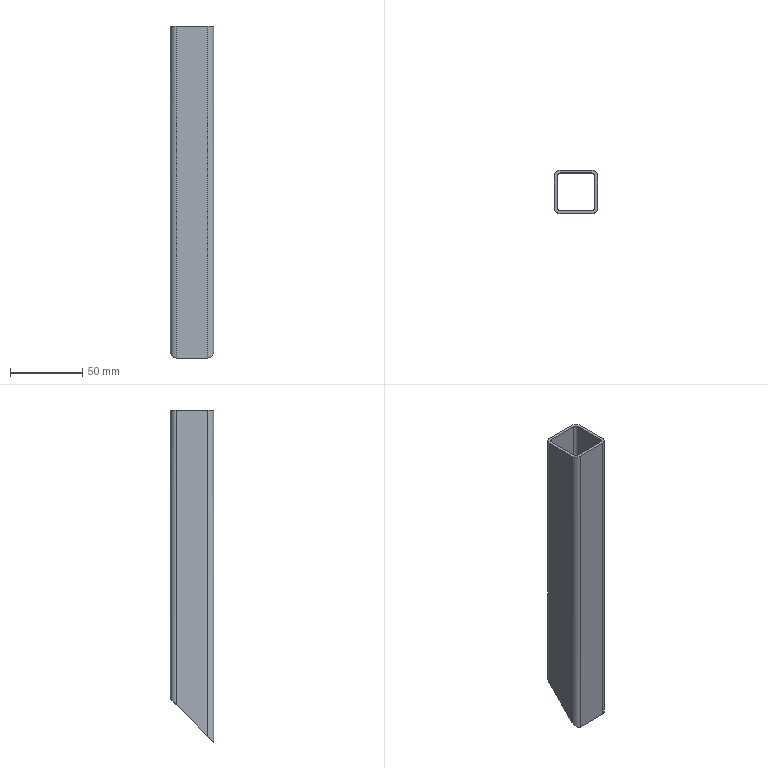Part | NX | features DATUM_CSYS 3, EXTRUDE 2, SKETCH 2, CPROJ 1 | 1 solid | 18 faces | box 30 x 30 x 230 mm | volume 45945 mm3 | plane 10 | cylinder 8 | commonest cylinder face diameters 4 x4 8 x4
STEP:
#1=CARTESIAN_POINT('',(15.,11.,230.));
#2=VERTEX_POINT('',#1);
#3=CARTESIAN_POINT('',(11.,15.,230.));
#4=VERTEX_POINT('',#3);
#5=CARTESIAN_POINT('',(11.,11.,230.));
#6=DIRECTION('',(0.,0.,1.));
#7=DIRECTION('',(1.,0.,0.));
#8=AXIS2_PLACEMENT_3D('',#5,#6,#7);
#9=CIRCLE('',#8,4.);
#10=EDGE_CURVE('',#2,#4,#9,.T.);
#11=ORIENTED_EDGE('',*,*,#10,.T.);
#12=CARTESIAN_POINT('',(-11.,15.,230.));
#13=VERTEX_POINT('',#12);
#14=CARTESIAN_POINT('',(11.,15.,230.));
#15=DIRECTION('',(-1.,0.,0.));
#16=VECTOR('',#15,1000.);
#17=LINE('',#14,#16);
#18=EDGE_CURVE('',#4,#13,#17,.T.);
#19=ORIENTED_EDGE('',*,*,#18,.T.);
#20=CARTESIAN_POINT('',(-15.,11.,230.));
#21=VERTEX_POINT('',#20);
#22=CARTESIAN_POINT('',(-11.,11.,230.));
#23=DIRECTION('',(0.,0.,1.));
#24=DIRECTION('',(1.,0.,0.));
#25=AXIS2_PLACEMENT_3D('',#22,#23,#24);
#26=CIRCLE('',#25,4.);
#27=EDGE_CURVE('',#13,#21,#26,.T.);
#28=ORIENTED_EDGE('',*,*,#27,.T.);
#29=CARTESIAN_POINT('',(-15.,-11.,230.));
#30=VERTEX_POINT('',#29);
#31=CARTESIAN_POINT('',(-15.,11.,230.));
#32=DIRECTION('',(0.,-1.,0.));
#33=VECTOR('',#32,1000.);
#34=LINE('',#31,#33);
#35=EDGE_CURVE('',#21,#30,#34,.T.);
#36=ORIENTED_EDGE('',*,*,#35,.T.);
#37=CARTESIAN_POINT('',(-11.,-15.,230.));
#38=VERTEX_POINT('',#37);
#39=CARTESIAN_POINT('',(-11.,-11.,230.));
#40=DIRECTION('',(0.,0.,1.));
#41=DIRECTION('',(1.,0.,0.));
#42=AXIS2_PLACEMENT_3D('',#39,#40,#41);
#43=CIRCLE('',#42,4.);
#44=EDGE_CURVE('',#30,#38,#43,.T.);
#45=ORIENTED_EDGE('',*,*,#44,.T.);
#46=CARTESIAN_POINT('',(11.,-15.,230.));
#47=VERTEX_POINT('',#46);
#48=CARTESIAN_POINT('',(-11.,-15.,230.));
#49=DIRECTION('',(1.,0.,0.));
#50=VECTOR('',#49,1000.);
#51=LINE('',#48,#50);
#52=EDGE_CURVE('',#38,#47,#51,.T.);
#53=ORIENTED_EDGE('',*,*,#52,.T.);
#54=CARTESIAN_POINT('',(15.,-11.,230.));
#55=VERTEX_POINT('',#54);
#56=CARTESIAN_POINT('',(11.,-11.,230.));
#57=DIRECTION('',(0.,0.,1.));
#58=DIRECTION('',(1.,0.,0.));
#59=AXIS2_PLACEMENT_3D('',#56,#57,#58);
#60=CIRCLE('',#59,4.);
#61=EDGE_CURVE('',#47,#55,#60,.T.);
#62=ORIENTED_EDGE('',*,*,#61,.T.);
#63=CARTESIAN_POINT('',(15.,-11.,230.));
#64=DIRECTION('',(0.,1.,0.));
#65=VECTOR('',#64,1000.);
#66=LINE('',#63,#65);
#67=EDGE_CURVE('',#55,#2,#66,.T.);
#68=ORIENTED_EDGE('',*,*,#67,.T.);
#69=EDGE_LOOP('',(#11,#19,#28,#36,#45,#53,#62,#68));
#70=FACE_BOUND('',#69,.T.);
#71=CARTESIAN_POINT('',(13.,11.,230.));
#72=VERTEX_POINT('',#71);
#73=CARTESIAN_POINT('',(11.,13.,230.));
#74=VERTEX_POINT('',#73);
#75=CARTESIAN_POINT('',(11.,11.,230.));
#76=DIRECTION('',(0.,0.,1.));
#77=DIRECTION('',(1.,0.,0.));
#78=AXIS2_PLACEMENT_3D('',#75,#76,#77);
#79=CIRCLE('',#78,2.);
#80=EDGE_CURVE('',#72,#74,#79,.T.);
#81=ORIENTED_EDGE('',*,*,#80,.F.);
#82=CARTESIAN_POINT('',(13.,-11.,230.));
#83=VERTEX_POINT('',#82);
#84=CARTESIAN_POINT('',(13.,-11.,230.));
#85=DIRECTION('',(0.,1.,0.));
#86=VECTOR('',#85,1000.);
#87=LINE('',#84,#86);
#88=EDGE_CURVE('',#83,#72,#87,.T.);
#89=ORIENTED_EDGE('',*,*,#88,.F.);
#90=CARTESIAN_POINT('',(11.,-13.,230.));
#91=VERTEX_POINT('',#90);
#92=CARTESIAN_POINT('',(11.,-11.,230.));
#93=DIRECTION('',(0.,0.,1.));
#94=DIRECTION('',(1.,0.,0.));
#95=AXIS2_PLACEMENT_3D('',#92,#93,#94);
#96=CIRCLE('',#95,2.);
#97=EDGE_CURVE('',#91,#83,#96,.T.);
#98=ORIENTED_EDGE('',*,*,#97,.F.);
#99=CARTESIAN_POINT('',(-11.,-13.,230.));
#100=VERTEX_POINT('',#99);
#101=CARTESIAN_POINT('',(-11.,-13.,230.));
#102=DIRECTION('',(1.,0.,0.));
#103=VECTOR('',#102,1000.);
#104=LINE('',#101,#103);
#105=EDGE_CURVE('',#100,#91,#104,.T.);
#106=ORIENTED_EDGE('',*,*,#105,.F.);
#107=CARTESIAN_POINT('',(-13.,-11.,230.));
#108=VERTEX_POINT('',#107);
#109=CARTESIAN_POINT('',(-11.,-11.,230.));
#110=DIRECTION('',(0.,0.,1.));
#111=DIRECTION('',(1.,0.,0.));
#112=AXIS2_PLACEMENT_3D('',#109,#110,#111);
#113=CIRCLE('',#112,2.);
#114=EDGE_CURVE('',#108,#100,#113,.T.);
#115=ORIENTED_EDGE('',*,*,#114,.F.);
#116=CARTESIAN_POINT('',(-13.,11.,230.));
#117=VERTEX_POINT('',#116);
#118=CARTESIAN_POINT('',(-13.,11.,230.));
#119=DIRECTION('',(0.,-1.,0.));
#120=VECTOR('',#119,1000.);
#121=LINE('',#118,#120);
#122=EDGE_CURVE('',#117,#108,#121,.T.);
#123=ORIENTED_EDGE('',*,*,#122,.F.);
#124=CARTESIAN_POINT('',(-11.,13.,230.));
#125=VERTEX_POINT('',#124);
#126=CARTESIAN_POINT('',(-11.,11.,230.));
#127=DIRECTION('',(0.,0.,1.));
#128=DIRECTION('',(1.,0.,0.));
#129=AXIS2_PLACEMENT_3D('',#126,#127,#128);
#130=CIRCLE('',#129,2.);
#131=EDGE_CURVE('',#125,#117,#130,.T.);
#132=ORIENTED_EDGE('',*,*,#131,.F.);
#133=CARTESIAN_POINT('',(11.,13.,230.));
#134=DIRECTION('',(-1.,0.,0.));
#135=VECTOR('',#134,1000.);
#136=LINE('',#133,#135);
#137=EDGE_CURVE('',#74,#125,#136,.T.);
#138=ORIENTED_EDGE('',*,*,#137,.F.);
#139=EDGE_LOOP('',(#81,#89,#98,#106,#115,#123,#132,#138));
#140=FACE_BOUND('',#139,.T.);
#141=CARTESIAN_POINT('',(11.,11.,230.));
#142=DIRECTION('',(0.,0.,-1.));
#143=DIRECTION('',(-1.,0.,0.));
#144=AXIS2_PLACEMENT_3D('',#141,#142,#143);
#145=PLANE('',#144);
#146=ADVANCED_FACE('',(#70,#140),#145,.F.);
#147=CARTESIAN_POINT('',(-11.,15.,30.));
#148=VERTEX_POINT('',#147);
#149=CARTESIAN_POINT('',(11.,15.,30.));
#150=VERTEX_POINT('',#149);
#151=CARTESIAN_POINT('',(-29.5,15.,30.));
#152=DIRECTION('',(1.,0.,0.));
#153=VECTOR('',#152,1000.);
#154=LINE('',#151,#153);
#155=EDGE_CURVE('',#148,#150,#154,.T.);
#156=ORIENTED_EDGE('',*,*,#155,.F.);
#157=CARTESIAN_POINT('',(-11.,15.,0.));
#158=DIRECTION('',(0.,0.,1.));
#159=VECTOR('',#158,1000.);
#160=LINE('',#157,#159);
#161=EDGE_CURVE('',#148,#13,#160,.T.);
#162=ORIENTED_EDGE('',*,*,#161,.T.);
#163=ORIENTED_EDGE('',*,*,#18,.F.);
#164=CARTESIAN_POINT('',(11.,15.,0.));
#165=DIRECTION('',(0.,0.,1.));
#166=VECTOR('',#165,1000.);
#167=LINE('',#164,#166);
#168=EDGE_CURVE('',#150,#4,#167,.T.);
#169=ORIENTED_EDGE('',*,*,#168,.F.);
#170=EDGE_LOOP('',(#156,#162,#163,#169));
#171=FACE_BOUND('',#170,.T.);
#172=CARTESIAN_POINT('',(11.,15.,0.));
#173=DIRECTION('',(0.,1.,0.));
#174=DIRECTION('',(-1.,0.,0.));
#175=AXIS2_PLACEMENT_3D('',#172,#173,#174);
#176=PLANE('',#175);
#177=ADVANCED_FACE('',(#171),#176,.T.);
#178=CARTESIAN_POINT('',(-15.,11.,26.));
#179=VERTEX_POINT('',#178);
#180=CARTESIAN_POINT('',(-11.,11.,26.));
#181=DIRECTION('',(0.,-0.7071,0.7071));
#182=DIRECTION('',(0.,0.7071,0.7071));
#183=AXIS2_PLACEMENT_3D('',#180,#181,#182);
#184=ELLIPSE('',#183,5.657,4.);
#185=EDGE_CURVE('',#179,#148,#184,.F.);
#186=ORIENTED_EDGE('',*,*,#185,.F.);
#187=CARTESIAN_POINT('',(-15.,11.,0.));
#188=DIRECTION('',(0.,0.,1.));
#189=VECTOR('',#188,1000.);
#190=LINE('',#187,#189);
#191=EDGE_CURVE('',#179,#21,#190,.T.);
#192=ORIENTED_EDGE('',*,*,#191,.T.);
#193=ORIENTED_EDGE('',*,*,#27,.F.);
#194=ORIENTED_EDGE('',*,*,#161,.F.);
#195=EDGE_LOOP('',(#186,#192,#193,#194));
#196=FACE_BOUND('',#195,.T.);
#197=CARTESIAN_POINT('',(-11.,11.,0.));
#198=DIRECTION('',(0.,0.,1.));
#199=DIRECTION('',(1.,0.,0.));
#200=AXIS2_PLACEMENT_3D('',#197,#198,#199);
#201=CYLINDRICAL_SURFACE('',#200,4.);
#202=ADVANCED_FACE('',(#196),#201,.T.);
#203=CARTESIAN_POINT('',(-15.,-11.,4.));
#204=VERTEX_POINT('',#203);
#205=CARTESIAN_POINT('',(-15.,-2.,13.));
#206=DIRECTION('',(0.,0.7071,0.7071));
#207=VECTOR('',#206,1000.);
#208=LINE('',#205,#207);
#209=EDGE_CURVE('',#204,#179,#208,.T.);
#210=ORIENTED_EDGE('',*,*,#209,.F.);
#211=CARTESIAN_POINT('',(-15.,-11.,0.));
#212=DIRECTION('',(0.,0.,1.));
#213=VECTOR('',#212,1000.);
#214=LINE('',#211,#213);
#215=EDGE_CURVE('',#204,#30,#214,.T.);
#216=ORIENTED_EDGE('',*,*,#215,.T.);
#217=ORIENTED_EDGE('',*,*,#35,.F.);
#218=ORIENTED_EDGE('',*,*,#191,.F.);
#219=EDGE_LOOP('',(#210,#216,#217,#218));
#220=FACE_BOUND('',#219,.T.);
#221=CARTESIAN_POINT('',(-15.,11.,0.));
#222=DIRECTION('',(-1.,0.,0.));
#223=DIRECTION('',(0.,-1.,0.));
#224=AXIS2_PLACEMENT_3D('',#221,#222,#223);
#225=PLANE('',#224);
#226=ADVANCED_FACE('',(#220),#225,.T.);
#227=CARTESIAN_POINT('',(-11.,-15.,0.));
#228=VERTEX_POINT('',#227);
#229=CARTESIAN_POINT('',(-11.,-11.,4.));
#230=DIRECTION('',(0.,-0.7071,0.7071));
#231=DIRECTION('',(0.,0.7071,0.7071));
#232=AXIS2_PLACEMENT_3D('',#229,#230,#231);
#233=ELLIPSE('',#232,5.657,4.);
#234=EDGE_CURVE('',#228,#204,#233,.F.);
#235=ORIENTED_EDGE('',*,*,#234,.F.);
#236=CARTESIAN_POINT('',(-11.,-15.,0.));
#237=DIRECTION('',(0.,0.,1.));
#238=VECTOR('',#237,1000.);
#239=LINE('',#236,#238);
#240=EDGE_CURVE('',#228,#38,#239,.T.);
#241=ORIENTED_EDGE('',*,*,#240,.T.);
#242=ORIENTED_EDGE('',*,*,#44,.F.);
#243=ORIENTED_EDGE('',*,*,#215,.F.);
#244=EDGE_LOOP('',(#235,#241,#242,#243));
#245=FACE_BOUND('',#244,.T.);
#246=CARTESIAN_POINT('',(-11.,-11.,0.));
#247=DIRECTION('',(0.,0.,1.));
#248=DIRECTION('',(1.,0.,0.));
#249=AXIS2_PLACEMENT_3D('',#246,#247,#248);
#250=CYLINDRICAL_SURFACE('',#249,4.);
#251=ADVANCED_FACE('',(#245),#250,.T.);
#252=ORIENTED_EDGE('',*,*,#52,.F.);
#253=ORIENTED_EDGE('',*,*,#240,.F.);
#254=CARTESIAN_POINT('',(11.,-15.,0.));
#255=VERTEX_POINT('',#254);
#256=CARTESIAN_POINT('',(-11.,-15.,0.));
#257=DIRECTION('',(1.,0.,0.));
#258=VECTOR('',#257,1000.);
#259=LINE('',#256,#258);
#260=EDGE_CURVE('',#228,#255,#259,.T.);
#261=ORIENTED_EDGE('',*,*,#260,.T.);
#262=CARTESIAN_POINT('',(11.,-15.,0.));
#263=DIRECTION('',(0.,0.,1.));
#264=VECTOR('',#263,1000.);
#265=LINE('',#262,#264);
#266=EDGE_CURVE('',#255,#47,#265,.T.);
#267=ORIENTED_EDGE('',*,*,#266,.T.);
#268=EDGE_LOOP('',(#252,#253,#261,#267));
#269=FACE_BOUND('',#268,.T.);
#270=CARTESIAN_POINT('',(-11.,-15.,0.));
#271=DIRECTION('',(0.,-1.,0.));
#272=DIRECTION('',(1.,0.,0.));
#273=AXIS2_PLACEMENT_3D('',#270,#271,#272);
#274=PLANE('',#273);
#275=ADVANCED_FACE('',(#269),#274,.T.);
#276=CARTESIAN_POINT('',(15.,-11.,4.));
#277=VERTEX_POINT('',#276);
#278=CARTESIAN_POINT('',(11.,-11.,4.));
#279=DIRECTION('',(0.,-0.7071,0.7071));
#280=DIRECTION('',(0.,0.7071,0.7071));
#281=AXIS2_PLACEMENT_3D('',#278,#279,#280);
#282=ELLIPSE('',#281,5.657,4.);
#283=EDGE_CURVE('',#277,#255,#282,.F.);
#284=ORIENTED_EDGE('',*,*,#283,.F.);
#285=CARTESIAN_POINT('',(15.,-11.,0.));
#286=DIRECTION('',(0.,0.,1.));
#287=VECTOR('',#286,1000.);
#288=LINE('',#285,#287);
#289=EDGE_CURVE('',#277,#55,#288,.T.);
#290=ORIENTED_EDGE('',*,*,#289,.T.);
#291=ORIENTED_EDGE('',*,*,#61,.F.);
#292=ORIENTED_EDGE('',*,*,#266,.F.);
#293=EDGE_LOOP('',(#284,#290,#291,#292));
#294=FACE_BOUND('',#293,.T.);
#295=CARTESIAN_POINT('',(11.,-11.,0.));
#296=DIRECTION('',(0.,0.,1.));
#297=DIRECTION('',(1.,0.,0.));
#298=AXIS2_PLACEMENT_3D('',#295,#296,#297);
#299=CYLINDRICAL_SURFACE('',#298,4.);
#300=ADVANCED_FACE('',(#294),#299,.T.);
#301=CARTESIAN_POINT('',(15.,11.,26.));
#302=VERTEX_POINT('',#301);
#303=CARTESIAN_POINT('',(15.,15.,30.));
#304=DIRECTION('',(0.,-0.7071,-0.7071));
#305=VECTOR('',#304,1000.);
#306=LINE('',#303,#305);
#307=EDGE_CURVE('',#302,#277,#306,.T.);
#308=ORIENTED_EDGE('',*,*,#307,.F.);
#309=CARTESIAN_POINT('',(15.,11.,0.));
#310=DIRECTION('',(0.,0.,1.));
#311=VECTOR('',#310,1000.);
#312=LINE('',#309,#311);
#313=EDGE_CURVE('',#302,#2,#312,.T.);
#314=ORIENTED_EDGE('',*,*,#313,.T.);
#315=ORIENTED_EDGE('',*,*,#67,.F.);
#316=ORIENTED_EDGE('',*,*,#289,.F.);
#317=EDGE_LOOP('',(#308,#314,#315,#316));
#318=FACE_BOUND('',#317,.T.);
#319=CARTESIAN_POINT('',(15.,-11.,0.));
#320=DIRECTION('',(1.,0.,0.));
#321=DIRECTION('',(0.,0.,-1.));
#322=AXIS2_PLACEMENT_3D('',#319,#320,#321);
#323=PLANE('',#322);
#324=ADVANCED_FACE('',(#318),#323,.T.);
#325=CARTESIAN_POINT('',(11.,11.,26.));
#326=DIRECTION('',(0.,-0.7071,0.7071));
#327=DIRECTION('',(0.,0.7071,0.7071));
#328=AXIS2_PLACEMENT_3D('',#325,#326,#327);
#329=ELLIPSE('',#328,5.657,4.);
#330=EDGE_CURVE('',#150,#302,#329,.F.);
#331=ORIENTED_EDGE('',*,*,#330,.F.);
#332=ORIENTED_EDGE('',*,*,#168,.T.);
#333=ORIENTED_EDGE('',*,*,#10,.F.);
#334=ORIENTED_EDGE('',*,*,#313,.F.);
#335=EDGE_LOOP('',(#331,#332,#333,#334));
#336=FACE_BOUND('',#335,.T.);
#337=CARTESIAN_POINT('',(11.,11.,0.));
#338=DIRECTION('',(0.,0.,1.));
#339=DIRECTION('',(1.,0.,0.));
#340=AXIS2_PLACEMENT_3D('',#337,#338,#339);
#341=CYLINDRICAL_SURFACE('',#340,4.);
#342=ADVANCED_FACE('',(#336),#341,.T.);
#343=CARTESIAN_POINT('',(-11.,13.,28.));
#344=VERTEX_POINT('',#343);
#345=CARTESIAN_POINT('',(-11.,13.,0.));
#346=DIRECTION('',(0.,0.,1.));
#347=VECTOR('',#346,1000.);
#348=LINE('',#345,#347);
#349=EDGE_CURVE('',#344,#125,#348,.T.);
#350=ORIENTED_EDGE('',*,*,#349,.F.);
#351=CARTESIAN_POINT('',(11.,13.,28.));
#352=VERTEX_POINT('',#351);
#353=CARTESIAN_POINT('',(11.,13.,28.));
#354=DIRECTION('',(1.,0.,0.));
#355=VECTOR('',#354,1000.);
#356=LINE('',#353,#355);
#357=EDGE_CURVE('',#344,#352,#356,.T.);
#358=ORIENTED_EDGE('',*,*,#357,.T.);
#359=CARTESIAN_POINT('',(11.,13.,0.));
#360=DIRECTION('',(0.,0.,1.));
#361=VECTOR('',#360,1000.);
#362=LINE('',#359,#361);
#363=EDGE_CURVE('',#352,#74,#362,.T.);
#364=ORIENTED_EDGE('',*,*,#363,.T.);
#365=ORIENTED_EDGE('',*,*,#137,.T.);
#366=EDGE_LOOP('',(#350,#358,#364,#365));
#367=FACE_BOUND('',#366,.T.);
#368=CARTESIAN_POINT('',(11.,13.,0.));
#369=DIRECTION('',(0.,1.,0.));
#370=DIRECTION('',(-1.,0.,0.));
#371=AXIS2_PLACEMENT_3D('',#368,#369,#370);
#372=PLANE('',#371);
#373=ADVANCED_FACE('',(#367),#372,.F.);
#374=CARTESIAN_POINT('',(-13.,11.,26.));
#375=VERTEX_POINT('',#374);
#376=CARTESIAN_POINT('',(-13.,11.,0.));
#377=DIRECTION('',(0.,0.,1.));
#378=VECTOR('',#377,1000.);
#379=LINE('',#376,#378);
#380=EDGE_CURVE('',#375,#117,#379,.T.);
#381=ORIENTED_EDGE('',*,*,#380,.F.);
#382=CARTESIAN_POINT('',(-11.,11.,26.));
#383=DIRECTION('',(0.,-0.7071,0.7071));
#384=DIRECTION('',(0.,0.7071,0.7071));
#385=AXIS2_PLACEMENT_3D('',#382,#383,#384);
#386=ELLIPSE('',#385,2.828,2.);
#387=EDGE_CURVE('',#375,#344,#386,.F.);
#388=ORIENTED_EDGE('',*,*,#387,.T.);
#389=ORIENTED_EDGE('',*,*,#349,.T.);
#390=ORIENTED_EDGE('',*,*,#131,.T.);
#391=EDGE_LOOP('',(#381,#388,#389,#390));
#392=FACE_BOUND('',#391,.T.);
#393=CARTESIAN_POINT('',(-11.,11.,0.));
#394=DIRECTION('',(0.,0.,1.));
#395=DIRECTION('',(1.,0.,0.));
#396=AXIS2_PLACEMENT_3D('',#393,#394,#395);
#397=CYLINDRICAL_SURFACE('',#396,2.);
#398=ADVANCED_FACE('',(#392),#397,.F.);
#399=CARTESIAN_POINT('',(-13.,-11.,4.));
#400=VERTEX_POINT('',#399);
#401=CARTESIAN_POINT('',(-13.,-11.,0.));
#402=DIRECTION('',(0.,0.,1.));
#403=VECTOR('',#402,1000.);
#404=LINE('',#401,#403);
#405=EDGE_CURVE('',#400,#108,#404,.T.);
#406=ORIENTED_EDGE('',*,*,#405,.F.);
#407=CARTESIAN_POINT('',(-13.,-2.,13.));
#408=DIRECTION('',(0.,0.7071,0.7071));
#409=VECTOR('',#408,1000.);
#410=LINE('',#407,#409);
#411=EDGE_CURVE('',#400,#375,#410,.T.);
#412=ORIENTED_EDGE('',*,*,#411,.T.);
#413=ORIENTED_EDGE('',*,*,#380,.T.);
#414=ORIENTED_EDGE('',*,*,#122,.T.);
#415=EDGE_LOOP('',(#406,#412,#413,#414));
#416=FACE_BOUND('',#415,.T.);
#417=CARTESIAN_POINT('',(-13.,11.,0.));
#418=DIRECTION('',(-1.,0.,0.));
#419=DIRECTION('',(0.,-1.,0.));
#420=AXIS2_PLACEMENT_3D('',#417,#418,#419);
#421=PLANE('',#420);
#422=ADVANCED_FACE('',(#416),#421,.F.);
#423=CARTESIAN_POINT('',(-11.,-13.,2.));
#424=VERTEX_POINT('',#423);
#425=CARTESIAN_POINT('',(-11.,-13.,0.));
#426=DIRECTION('',(0.,0.,1.));
#427=VECTOR('',#426,1000.);
#428=LINE('',#425,#427);
#429=EDGE_CURVE('',#424,#100,#428,.T.);
#430=ORIENTED_EDGE('',*,*,#429,.F.);
#431=CARTESIAN_POINT('',(-11.,-11.,4.));
#432=DIRECTION('',(0.,-0.7071,0.7071));
#433=DIRECTION('',(0.,0.7071,0.7071));
#434=AXIS2_PLACEMENT_3D('',#431,#432,#433);
#435=ELLIPSE('',#434,2.828,2.);
#436=EDGE_CURVE('',#424,#400,#435,.F.);
#437=ORIENTED_EDGE('',*,*,#436,.T.);
#438=ORIENTED_EDGE('',*,*,#405,.T.);
#439=ORIENTED_EDGE('',*,*,#114,.T.);
#440=EDGE_LOOP('',(#430,#437,#438,#439));
#441=FACE_BOUND('',#440,.T.);
#442=CARTESIAN_POINT('',(-11.,-11.,0.));
#443=DIRECTION('',(0.,0.,1.));
#444=DIRECTION('',(1.,0.,0.));
#445=AXIS2_PLACEMENT_3D('',#442,#443,#444);
#446=CYLINDRICAL_SURFACE('',#445,2.);
#447=ADVANCED_FACE('',(#441),#446,.F.);
#448=CARTESIAN_POINT('',(11.,-13.,2.));
#449=VERTEX_POINT('',#448);
#450=CARTESIAN_POINT('',(11.,-13.,0.));
#451=DIRECTION('',(0.,0.,1.));
#452=VECTOR('',#451,1000.);
#453=LINE('',#450,#452);
#454=EDGE_CURVE('',#449,#91,#453,.T.);
#455=ORIENTED_EDGE('',*,*,#454,.F.);
#456=CARTESIAN_POINT('',(-11.,-13.,2.));
#457=DIRECTION('',(-1.,0.,0.));
#458=VECTOR('',#457,1000.);
#459=LINE('',#456,#458);
#460=EDGE_CURVE('',#449,#424,#459,.T.);
#461=ORIENTED_EDGE('',*,*,#460,.T.);
#462=ORIENTED_EDGE('',*,*,#429,.T.);
#463=ORIENTED_EDGE('',*,*,#105,.T.);
#464=EDGE_LOOP('',(#455,#461,#462,#463));
#465=FACE_BOUND('',#464,.T.);
#466=CARTESIAN_POINT('',(-11.,-13.,0.));
#467=DIRECTION('',(0.,-1.,0.));
#468=DIRECTION('',(1.,0.,0.));
#469=AXIS2_PLACEMENT_3D('',#466,#467,#468);
#470=PLANE('',#469);
#471=ADVANCED_FACE('',(#465),#470,.F.);
#472=CARTESIAN_POINT('',(13.,-11.,4.));
#473=VERTEX_POINT('',#472);
#474=CARTESIAN_POINT('',(13.,-11.,0.));
#475=DIRECTION('',(0.,0.,1.));
#476=VECTOR('',#475,1000.);
#477=LINE('',#474,#476);
#478=EDGE_CURVE('',#473,#83,#477,.T.);
#479=ORIENTED_EDGE('',*,*,#478,.F.);
#480=CARTESIAN_POINT('',(11.,-11.,4.));
#481=DIRECTION('',(0.,-0.7071,0.7071));
#482=DIRECTION('',(0.,0.7071,0.7071));
#483=AXIS2_PLACEMENT_3D('',#480,#481,#482);
#484=ELLIPSE('',#483,2.828,2.);
#485=EDGE_CURVE('',#473,#449,#484,.F.);
#486=ORIENTED_EDGE('',*,*,#485,.T.);
#487=ORIENTED_EDGE('',*,*,#454,.T.);
#488=ORIENTED_EDGE('',*,*,#97,.T.);
#489=EDGE_LOOP('',(#479,#486,#487,#488));
#490=FACE_BOUND('',#489,.T.);
#491=CARTESIAN_POINT('',(11.,-11.,0.));
#492=DIRECTION('',(0.,0.,1.));
#493=DIRECTION('',(1.,0.,0.));
#494=AXIS2_PLACEMENT_3D('',#491,#492,#493);
#495=CYLINDRICAL_SURFACE('',#494,2.);
#496=ADVANCED_FACE('',(#490),#495,.F.);
#497=CARTESIAN_POINT('',(13.,11.,26.));
#498=VERTEX_POINT('',#497);
#499=CARTESIAN_POINT('',(13.,11.,0.));
#500=DIRECTION('',(0.,0.,-1.));
#501=VECTOR('',#500,1000.);
#502=LINE('',#499,#501);
#503=EDGE_CURVE('',#498,#72,#502,.F.);
#504=ORIENTED_EDGE('',*,*,#503,.F.);
#505=CARTESIAN_POINT('',(13.,-13.,2.));
#506=DIRECTION('',(0.,-0.7071,-0.7071));
#507=VECTOR('',#506,1000.);
#508=LINE('',#505,#507);
#509=EDGE_CURVE('',#498,#473,#508,.T.);
#510=ORIENTED_EDGE('',*,*,#509,.T.);
#511=ORIENTED_EDGE('',*,*,#478,.T.);
#512=ORIENTED_EDGE('',*,*,#88,.T.);
#513=EDGE_LOOP('',(#504,#510,#511,#512));
#514=FACE_BOUND('',#513,.T.);
#515=CARTESIAN_POINT('',(13.,-11.,0.));
#516=DIRECTION('',(1.,0.,0.));
#517=DIRECTION('',(0.,0.,-1.));
#518=AXIS2_PLACEMENT_3D('',#515,#516,#517);
#519=PLANE('',#518);
#520=ADVANCED_FACE('',(#514),#519,.F.);
#521=ORIENTED_EDGE('',*,*,#363,.F.);
#522=CARTESIAN_POINT('',(11.,11.,26.));
#523=DIRECTION('',(0.,-0.7071,0.7071));
#524=DIRECTION('',(0.,0.7071,0.7071));
#525=AXIS2_PLACEMENT_3D('',#522,#523,#524);
#526=ELLIPSE('',#525,2.828,2.);
#527=EDGE_CURVE('',#352,#498,#526,.F.);
#528=ORIENTED_EDGE('',*,*,#527,.T.);
#529=ORIENTED_EDGE('',*,*,#503,.T.);
#530=ORIENTED_EDGE('',*,*,#80,.T.);
#531=EDGE_LOOP('',(#521,#528,#529,#530));
#532=FACE_BOUND('',#531,.T.);
#533=CARTESIAN_POINT('',(11.,11.,0.));
#534=DIRECTION('',(0.,0.,1.));
#535=DIRECTION('',(1.,0.,0.));
#536=AXIS2_PLACEMENT_3D('',#533,#534,#535);
#537=CYLINDRICAL_SURFACE('',#536,2.);
#538=ADVANCED_FACE('',(#532),#537,.F.);
#539=ORIENTED_EDGE('',*,*,#185,.T.);
#540=ORIENTED_EDGE('',*,*,#155,.T.);
#541=ORIENTED_EDGE('',*,*,#330,.T.);
#542=ORIENTED_EDGE('',*,*,#307,.T.);
#543=ORIENTED_EDGE('',*,*,#283,.T.);
#544=ORIENTED_EDGE('',*,*,#260,.F.);
#545=ORIENTED_EDGE('',*,*,#234,.T.);
#546=ORIENTED_EDGE('',*,*,#209,.T.);
#547=EDGE_LOOP('',(#539,#540,#541,#542,#543,#544,#545,#546));
#548=FACE_BOUND('',#547,.T.);
#549=ORIENTED_EDGE('',*,*,#387,.F.);
#550=ORIENTED_EDGE('',*,*,#411,.F.);
#551=ORIENTED_EDGE('',*,*,#436,.F.);
#552=ORIENTED_EDGE('',*,*,#460,.F.);
#553=ORIENTED_EDGE('',*,*,#485,.F.);
#554=ORIENTED_EDGE('',*,*,#509,.F.);
#555=ORIENTED_EDGE('',*,*,#527,.F.);
#556=ORIENTED_EDGE('',*,*,#357,.F.);
#557=EDGE_LOOP('',(#549,#550,#551,#552,#553,#554,#555,#556));
#558=FACE_BOUND('',#557,.T.);
#559=CARTESIAN_POINT('',(-29.5,15.,30.));
#560=DIRECTION('',(0.,-0.7071,0.7071));
#561=DIRECTION('',(0.,-0.7071,-0.7071));
#562=AXIS2_PLACEMENT_3D('',#559,#560,#561);
#563=PLANE('',#562);
#564=ADVANCED_FACE('',(#548,#558),#563,.F.);
#565=CLOSED_SHELL('',(#146,#177,#202,#226,#251,#275,#300,#324,#342,#373,#398,#422,#447,#471,#496,#520,#538,#564));
#566=MANIFOLD_SOLID_BREP('',#565);
#567=(LENGTH_UNIT()NAMED_UNIT(*)SI_UNIT(.MILLI.,.METRE.));
#568=UNCERTAINTY_MEASURE_WITH_UNIT(LENGTH_MEASURE(0.00001),#567,'','');
#569=(NAMED_UNIT(*)PLANE_ANGLE_UNIT()SI_UNIT($,.RADIAN.));
#570=(NAMED_UNIT(*)SI_UNIT($,.STERADIAN.)SOLID_ANGLE_UNIT());
#571=(GEOMETRIC_REPRESENTATION_CONTEXT(3)GLOBAL_UNCERTAINTY_ASSIGNED_CONTEXT((#568))GLOBAL_UNIT_ASSIGNED_CONTEXT((#567,#569,#570))REPRESENTATION_CONTEXT('',''));
#572=ADVANCED_BREP_SHAPE_REPRESENTATION('',(#566),#571);